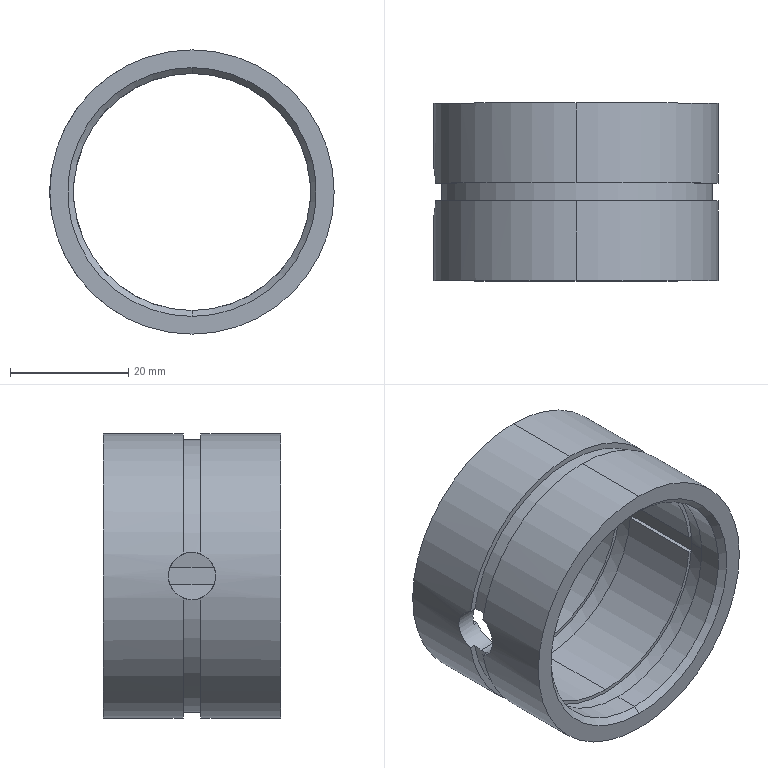Part | SolidWorks | features ICE 2, Chamfer 1, Extrusion 1, RevCut 1 | 1 solid | 49 faces | box 48 x 30 x 48 mm | volume 15342 mm3 | plane 27 | cylinder 18 | cone 4 | commonest cylinder face diameters 40 x7 41.2 x4 48 x4 8 x2 46 x1